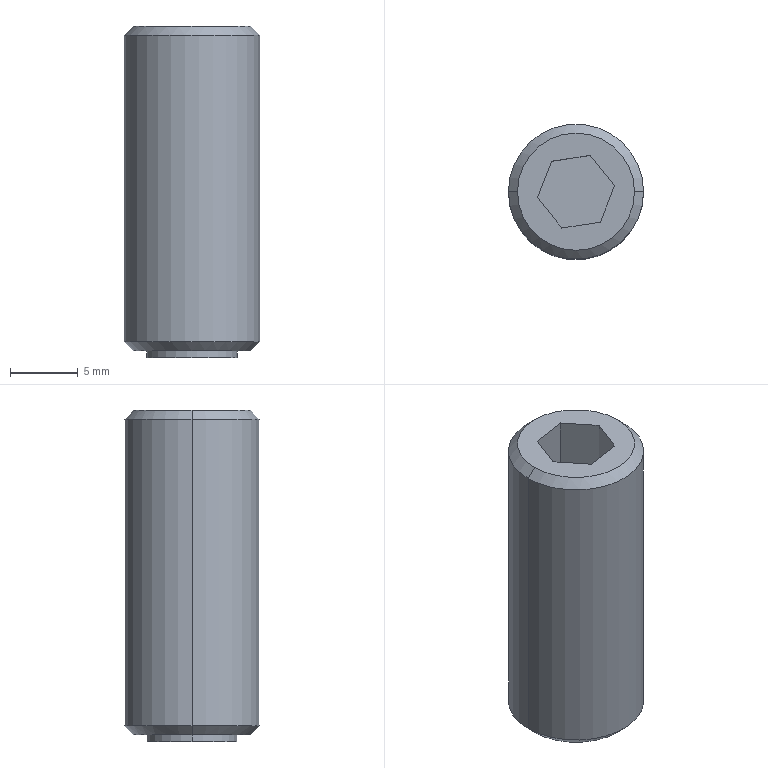Part | NX | 1 solid | 18 faces | box 10 x 10 x 24.5 mm | volume 1781 mm3 | plane 10 | cylinder 4 | cone 4 | commonest cylinder face diameters 6.667 x2 10 x2
STEP:
#1=CARTESIAN_POINT('',(3.333,0.,-12.5));
#2=VERTEX_POINT('',#1);
#3=CARTESIAN_POINT('',(-3.333,0.,-12.5));
#4=VERTEX_POINT('',#3);
#5=CARTESIAN_POINT('',(0.,0.,-12.5));
#6=DIRECTION('',(0.,0.,-1.));
#7=DIRECTION('',(-1.,0.,0.));
#8=AXIS2_PLACEMENT_3D('',#5,#6,#7);
#9=CIRCLE('',#8,3.333);
#10=EDGE_CURVE('',#2,#4,#9,.T.);
#11=ORIENTED_EDGE('',*,*,#10,.F.);
#12=CARTESIAN_POINT('',(3.333,0.,-12.));
#13=VERTEX_POINT('',#12);
#14=CARTESIAN_POINT('',(3.333,0.,-12.5));
#15=DIRECTION('',(0.,0.,1.));
#16=VECTOR('',#15,1000.);
#17=LINE('',#14,#16);
#18=EDGE_CURVE('',#2,#13,#17,.T.);
#19=ORIENTED_EDGE('',*,*,#18,.T.);
#20=CARTESIAN_POINT('',(-3.333,0.,-12.));
#21=VERTEX_POINT('',#20);
#22=CARTESIAN_POINT('',(0.,0.,-12.));
#23=DIRECTION('',(0.,0.,-1.));
#24=DIRECTION('',(1.,0.,0.));
#25=AXIS2_PLACEMENT_3D('',#22,#23,#24);
#26=CIRCLE('',#25,3.333);
#27=EDGE_CURVE('',#13,#21,#26,.T.);
#28=ORIENTED_EDGE('',*,*,#27,.T.);
#29=CARTESIAN_POINT('',(-3.333,0.,-12.5));
#30=DIRECTION('',(0.,0.,1.));
#31=VECTOR('',#30,1000.);
#32=LINE('',#29,#31);
#33=EDGE_CURVE('',#4,#21,#32,.T.);
#34=ORIENTED_EDGE('',*,*,#33,.F.);
#35=EDGE_LOOP('',(#11,#19,#28,#34));
#36=FACE_BOUND('',#35,.T.);
#37=CARTESIAN_POINT('',(0.,0.,-12.5));
#38=DIRECTION('',(0.,0.,1.));
#39=DIRECTION('',(1.,0.,0.));
#40=AXIS2_PLACEMENT_3D('',#37,#38,#39);
#41=CYLINDRICAL_SURFACE('',#40,3.333);
#42=ADVANCED_FACE('',(#36),#41,.T.);
#43=CARTESIAN_POINT('',(5.,0.,-11.333));
#44=VERTEX_POINT('',#43);
#45=CARTESIAN_POINT('',(-5.,0.,-11.333));
#46=VERTEX_POINT('',#45);
#47=CARTESIAN_POINT('',(0.,0.,-11.333));
#48=DIRECTION('',(0.,0.,1.));
#49=DIRECTION('',(1.,0.,0.));
#50=AXIS2_PLACEMENT_3D('',#47,#48,#49);
#51=CIRCLE('',#50,5.);
#52=EDGE_CURVE('',#44,#46,#51,.T.);
#53=ORIENTED_EDGE('',*,*,#52,.F.);
#54=CARTESIAN_POINT('',(4.333,0.,-12.));
#55=VERTEX_POINT('',#54);
#56=CARTESIAN_POINT('',(5.,0.,-11.333));
#57=DIRECTION('',(0.7071,0.,0.7071));
#58=VECTOR('',#57,1000.);
#59=LINE('',#56,#58);
#60=EDGE_CURVE('',#55,#44,#59,.T.);
#61=ORIENTED_EDGE('',*,*,#60,.F.);
#62=CARTESIAN_POINT('',(-4.333,0.,-12.));
#63=VERTEX_POINT('',#62);
#64=CARTESIAN_POINT('',(0.,0.,-12.));
#65=DIRECTION('',(0.,0.,-1.));
#66=DIRECTION('',(1.,0.,0.));
#67=AXIS2_PLACEMENT_3D('',#64,#65,#66);
#68=CIRCLE('',#67,4.333);
#69=EDGE_CURVE('',#63,#55,#68,.T.);
#70=ORIENTED_EDGE('',*,*,#69,.F.);
#71=CARTESIAN_POINT('',(-5.,0.,-11.333));
#72=DIRECTION('',(-0.7071,0.,0.7071));
#73=VECTOR('',#72,1000.);
#74=LINE('',#71,#73);
#75=EDGE_CURVE('',#63,#46,#74,.T.);
#76=ORIENTED_EDGE('',*,*,#75,.T.);
#77=EDGE_LOOP('',(#53,#61,#70,#76));
#78=FACE_BOUND('',#77,.T.);
#79=CARTESIAN_POINT('',(0.,0.,-11.333));
#80=DIRECTION('',(0.,0.,1.));
#81=DIRECTION('',(1.,0.,0.));
#82=AXIS2_PLACEMENT_3D('',#79,#80,#81);
#83=CONICAL_SURFACE('',#82,5.,0.7854);
#84=ADVANCED_FACE('',(#78),#83,.T.);
#85=CARTESIAN_POINT('',(4.333,0.,12.));
#86=VERTEX_POINT('',#85);
#87=CARTESIAN_POINT('',(-4.333,0.,12.));
#88=VERTEX_POINT('',#87);
#89=CARTESIAN_POINT('',(0.,0.,12.));
#90=DIRECTION('',(0.,0.,1.));
#91=DIRECTION('',(1.,0.,0.));
#92=AXIS2_PLACEMENT_3D('',#89,#90,#91);
#93=CIRCLE('',#92,4.333);
#94=EDGE_CURVE('',#86,#88,#93,.T.);
#95=ORIENTED_EDGE('',*,*,#94,.F.);
#96=CARTESIAN_POINT('',(5.,0.,11.333));
#97=VERTEX_POINT('',#96);
#98=CARTESIAN_POINT('',(4.333,0.,12.));
#99=DIRECTION('',(0.7071,0.,-0.7071));
#100=VECTOR('',#99,1000.);
#101=LINE('',#98,#100);
#102=EDGE_CURVE('',#86,#97,#101,.T.);
#103=ORIENTED_EDGE('',*,*,#102,.T.);
#104=CARTESIAN_POINT('',(-5.,0.,11.333));
#105=VERTEX_POINT('',#104);
#106=CARTESIAN_POINT('',(0.,0.,11.333));
#107=DIRECTION('',(0.,0.,-1.));
#108=DIRECTION('',(1.,0.,0.));
#109=AXIS2_PLACEMENT_3D('',#106,#107,#108);
#110=CIRCLE('',#109,5.);
#111=EDGE_CURVE('',#105,#97,#110,.T.);
#112=ORIENTED_EDGE('',*,*,#111,.F.);
#113=CARTESIAN_POINT('',(-4.333,0.,12.));
#114=DIRECTION('',(-0.7071,0.,-0.7071));
#115=VECTOR('',#114,1000.);
#116=LINE('',#113,#115);
#117=EDGE_CURVE('',#88,#105,#116,.T.);
#118=ORIENTED_EDGE('',*,*,#117,.F.);
#119=EDGE_LOOP('',(#95,#103,#112,#118));
#120=FACE_BOUND('',#119,.T.);
#121=CARTESIAN_POINT('',(0.,0.,12.));
#122=DIRECTION('',(0.,0.,-1.));
#123=DIRECTION('',(-1.,0.,0.));
#124=AXIS2_PLACEMENT_3D('',#121,#122,#123);
#125=CONICAL_SURFACE('',#124,4.333,0.7854);
#126=ADVANCED_FACE('',(#120),#125,.T.);
#127=CARTESIAN_POINT('',(0.,0.,11.333));
#128=DIRECTION('',(0.,0.,-1.));
#129=DIRECTION('',(1.,0.,0.));
#130=AXIS2_PLACEMENT_3D('',#127,#128,#129);
#131=CIRCLE('',#130,5.);
#132=EDGE_CURVE('',#97,#105,#131,.T.);
#133=ORIENTED_EDGE('',*,*,#132,.T.);
#134=CARTESIAN_POINT('',(-5.,0.,12.));
#135=DIRECTION('',(0.,0.,-1.));
#136=VECTOR('',#135,1000.);
#137=LINE('',#134,#136);
#138=EDGE_CURVE('',#46,#105,#137,.F.);
#139=ORIENTED_EDGE('',*,*,#138,.F.);
#140=CARTESIAN_POINT('',(0.,0.,-11.333));
#141=DIRECTION('',(0.,0.,1.));
#142=DIRECTION('',(1.,0.,0.));
#143=AXIS2_PLACEMENT_3D('',#140,#141,#142);
#144=CIRCLE('',#143,5.);
#145=EDGE_CURVE('',#46,#44,#144,.T.);
#146=ORIENTED_EDGE('',*,*,#145,.T.);
#147=CARTESIAN_POINT('',(5.,0.,12.));
#148=DIRECTION('',(0.,0.,-1.));
#149=VECTOR('',#148,1000.);
#150=LINE('',#147,#149);
#151=EDGE_CURVE('',#44,#97,#150,.F.);
#152=ORIENTED_EDGE('',*,*,#151,.T.);
#153=EDGE_LOOP('',(#133,#139,#146,#152));
#154=FACE_BOUND('',#153,.T.);
#155=CARTESIAN_POINT('',(0.,0.,12.));
#156=DIRECTION('',(0.,0.,-1.));
#157=DIRECTION('',(-1.,0.,0.));
#158=AXIS2_PLACEMENT_3D('',#155,#156,#157);
#159=CYLINDRICAL_SURFACE('',#158,5.);
#160=ADVANCED_FACE('',(#154),#159,.T.);
#161=ORIENTED_EDGE('',*,*,#69,.T.);
#162=CARTESIAN_POINT('',(0.,0.,-12.));
#163=DIRECTION('',(0.,0.,-1.));
#164=DIRECTION('',(1.,0.,0.));
#165=AXIS2_PLACEMENT_3D('',#162,#163,#164);
#166=CIRCLE('',#165,4.333);
#167=EDGE_CURVE('',#55,#63,#166,.T.);
#168=ORIENTED_EDGE('',*,*,#167,.T.);
#169=EDGE_LOOP('',(#161,#168));
#170=FACE_BOUND('',#169,.T.);
#171=CARTESIAN_POINT('',(0.,0.,-12.));
#172=DIRECTION('',(0.,0.,-1.));
#173=DIRECTION('',(1.,0.,0.));
#174=AXIS2_PLACEMENT_3D('',#171,#172,#173);
#175=CIRCLE('',#174,3.333);
#176=EDGE_CURVE('',#21,#13,#175,.T.);
#177=ORIENTED_EDGE('',*,*,#176,.F.);
#178=ORIENTED_EDGE('',*,*,#27,.F.);
#179=EDGE_LOOP('',(#177,#178));
#180=FACE_BOUND('',#179,.T.);
#181=CARTESIAN_POINT('',(0.,0.,-12.));
#182=DIRECTION('',(0.,0.,1.));
#183=DIRECTION('',(1.,0.,0.));
#184=AXIS2_PLACEMENT_3D('',#181,#182,#183);
#185=PLANE('',#184);
#186=ADVANCED_FACE('',(#170,#180),#185,.F.);
#187=CARTESIAN_POINT('',(-1.047,-2.69,7.));
#188=VERTEX_POINT('',#187);
#189=CARTESIAN_POINT('',(1.806,-2.252,7.));
#190=VERTEX_POINT('',#189);
#191=CARTESIAN_POINT('',(-1.047,-2.69,7.));
#192=DIRECTION('',(0.9884,0.1519,0.));
#193=VECTOR('',#192,1000.);
#194=LINE('',#191,#193);
#195=EDGE_CURVE('',#188,#190,#194,.T.);
#196=ORIENTED_EDGE('',*,*,#195,.T.);
#197=CARTESIAN_POINT('',(2.853,0.4385,7.));
#198=VERTEX_POINT('',#197);
#199=CARTESIAN_POINT('',(1.806,-2.252,7.));
#200=DIRECTION('',(0.3627,0.9319,0.));
#201=VECTOR('',#200,1000.);
#202=LINE('',#199,#201);
#203=EDGE_CURVE('',#190,#198,#202,.T.);
#204=ORIENTED_EDGE('',*,*,#203,.T.);
#205=CARTESIAN_POINT('',(1.047,2.69,7.));
#206=VERTEX_POINT('',#205);
#207=CARTESIAN_POINT('',(2.853,0.4385,7.));
#208=DIRECTION('',(-0.6257,0.78,0.));
#209=VECTOR('',#208,1000.);
#210=LINE('',#207,#209);
#211=EDGE_CURVE('',#198,#206,#210,.T.);
#212=ORIENTED_EDGE('',*,*,#211,.T.);
#213=CARTESIAN_POINT('',(-1.806,2.252,7.));
#214=VERTEX_POINT('',#213);
#215=CARTESIAN_POINT('',(1.047,2.69,7.));
#216=DIRECTION('',(-0.9884,-0.1519,0.));
#217=VECTOR('',#216,1000.);
#218=LINE('',#215,#217);
#219=EDGE_CURVE('',#206,#214,#218,.T.);
#220=ORIENTED_EDGE('',*,*,#219,.T.);
#221=CARTESIAN_POINT('',(-2.853,-0.4385,7.));
#222=VERTEX_POINT('',#221);
#223=CARTESIAN_POINT('',(-1.806,2.252,7.));
#224=DIRECTION('',(-0.3627,-0.9319,0.));
#225=VECTOR('',#224,1000.);
#226=LINE('',#223,#225);
#227=EDGE_CURVE('',#214,#222,#226,.T.);
#228=ORIENTED_EDGE('',*,*,#227,.T.);
#229=CARTESIAN_POINT('',(-2.853,-0.4385,7.));
#230=DIRECTION('',(0.6257,-0.78,0.));
#231=VECTOR('',#230,1000.);
#232=LINE('',#229,#231);
#233=EDGE_CURVE('',#222,#188,#232,.T.);
#234=ORIENTED_EDGE('',*,*,#233,.T.);
#235=EDGE_LOOP('',(#196,#204,#212,#220,#228,#234));
#236=FACE_BOUND('',#235,.T.);
#237=CARTESIAN_POINT('',(1.806,-2.252,7.));
#238=DIRECTION('',(0.,0.,1.));
#239=DIRECTION('',(1.,0.,0.));
#240=AXIS2_PLACEMENT_3D('',#237,#238,#239);
#241=PLANE('',#240);
#242=ADVANCED_FACE('',(#236),#241,.T.);
#243=ORIENTED_EDGE('',*,*,#94,.T.);
#244=CARTESIAN_POINT('',(0.,0.,12.));
#245=DIRECTION('',(0.,0.,1.));
#246=DIRECTION('',(1.,0.,0.));
#247=AXIS2_PLACEMENT_3D('',#244,#245,#246);
#248=CIRCLE('',#247,4.333);
#249=EDGE_CURVE('',#88,#86,#248,.T.);
#250=ORIENTED_EDGE('',*,*,#249,.T.);
#251=EDGE_LOOP('',(#243,#250));
#252=FACE_BOUND('',#251,.T.);
#253=CARTESIAN_POINT('',(-1.047,-2.69,12.));
#254=VERTEX_POINT('',#253);
#255=CARTESIAN_POINT('',(1.806,-2.252,12.));
#256=VERTEX_POINT('',#255);
#257=CARTESIAN_POINT('',(-1.047,-2.69,12.));
#258=DIRECTION('',(0.9884,0.1519,0.));
#259=VECTOR('',#258,1000.);
#260=LINE('',#257,#259);
#261=EDGE_CURVE('',#254,#256,#260,.T.);
#262=ORIENTED_EDGE('',*,*,#261,.F.);
#263=CARTESIAN_POINT('',(-2.853,-0.4385,12.));
#264=VERTEX_POINT('',#263);
#265=CARTESIAN_POINT('',(-2.853,-0.4385,12.));
#266=DIRECTION('',(0.6257,-0.78,0.));
#267=VECTOR('',#266,1000.);
#268=LINE('',#265,#267);
#269=EDGE_CURVE('',#264,#254,#268,.T.);
#270=ORIENTED_EDGE('',*,*,#269,.F.);
#271=CARTESIAN_POINT('',(-1.806,2.252,12.));
#272=VERTEX_POINT('',#271);
#273=CARTESIAN_POINT('',(-1.806,2.252,12.));
#274=DIRECTION('',(-0.3627,-0.9319,0.));
#275=VECTOR('',#274,1000.);
#276=LINE('',#273,#275);
#277=EDGE_CURVE('',#272,#264,#276,.T.);
#278=ORIENTED_EDGE('',*,*,#277,.F.);
#279=CARTESIAN_POINT('',(1.047,2.69,12.));
#280=VERTEX_POINT('',#279);
#281=CARTESIAN_POINT('',(1.047,2.69,12.));
#282=DIRECTION('',(-0.9884,-0.1519,0.));
#283=VECTOR('',#282,1000.);
#284=LINE('',#281,#283);
#285=EDGE_CURVE('',#280,#272,#284,.T.);
#286=ORIENTED_EDGE('',*,*,#285,.F.);
#287=CARTESIAN_POINT('',(2.853,0.4385,12.));
#288=VERTEX_POINT('',#287);
#289=CARTESIAN_POINT('',(2.853,0.4385,12.));
#290=DIRECTION('',(-0.6257,0.78,0.));
#291=VECTOR('',#290,1000.);
#292=LINE('',#289,#291);
#293=EDGE_CURVE('',#288,#280,#292,.T.);
#294=ORIENTED_EDGE('',*,*,#293,.F.);
#295=CARTESIAN_POINT('',(1.806,-2.252,12.));
#296=DIRECTION('',(0.3627,0.9319,0.));
#297=VECTOR('',#296,1000.);
#298=LINE('',#295,#297);
#299=EDGE_CURVE('',#256,#288,#298,.T.);
#300=ORIENTED_EDGE('',*,*,#299,.F.);
#301=EDGE_LOOP('',(#262,#270,#278,#286,#294,#300));
#302=FACE_BOUND('',#301,.T.);
#303=CARTESIAN_POINT('',(0.,0.,12.));
#304=DIRECTION('',(0.,0.,1.));
#305=DIRECTION('',(1.,0.,0.));
#306=AXIS2_PLACEMENT_3D('',#303,#304,#305);
#307=PLANE('',#306);
#308=ADVANCED_FACE('',(#252,#302),#307,.T.);
#309=ORIENTED_EDGE('',*,*,#10,.T.);
#310=CARTESIAN_POINT('',(0.,0.,-12.5));
#311=DIRECTION('',(0.,0.,-1.));
#312=DIRECTION('',(-1.,0.,0.));
#313=AXIS2_PLACEMENT_3D('',#310,#311,#312);
#314=CIRCLE('',#313,3.333);
#315=EDGE_CURVE('',#4,#2,#314,.T.);
#316=ORIENTED_EDGE('',*,*,#315,.T.);
#317=EDGE_LOOP('',(#309,#316));
#318=FACE_BOUND('',#317,.T.);
#319=CARTESIAN_POINT('',(0.,0.,-12.5));
#320=DIRECTION('',(0.,0.,-1.));
#321=DIRECTION('',(0.,-1.,0.));
#322=AXIS2_PLACEMENT_3D('',#319,#320,#321);
#323=PLANE('',#322);
#324=ADVANCED_FACE('',(#318),#323,.T.);
#325=ORIENTED_EDGE('',*,*,#299,.T.);
#326=CARTESIAN_POINT('',(2.853,0.4385,7.));
#327=DIRECTION('',(0.,0.,1.));
#328=VECTOR('',#327,1000.);
#329=LINE('',#326,#328);
#330=EDGE_CURVE('',#198,#288,#329,.T.);
#331=ORIENTED_EDGE('',*,*,#330,.F.);
#332=ORIENTED_EDGE('',*,*,#203,.F.);
#333=CARTESIAN_POINT('',(1.806,-2.252,7.));
#334=DIRECTION('',(0.,0.,1.));
#335=VECTOR('',#334,1000.);
#336=LINE('',#333,#335);
#337=EDGE_CURVE('',#190,#256,#336,.T.);
#338=ORIENTED_EDGE('',*,*,#337,.T.);
#339=EDGE_LOOP('',(#325,#331,#332,#338));
#340=FACE_BOUND('',#339,.T.);
#341=CARTESIAN_POINT('',(1.806,-2.252,7.));
#342=DIRECTION('',(0.9319,-0.3627,0.));
#343=DIRECTION('',(0.,0.,-1.));
#344=AXIS2_PLACEMENT_3D('',#341,#342,#343);
#345=PLANE('',#344);
#346=ADVANCED_FACE('',(#340),#345,.F.);
#347=ORIENTED_EDGE('',*,*,#261,.T.);
#348=ORIENTED_EDGE('',*,*,#337,.F.);
#349=ORIENTED_EDGE('',*,*,#195,.F.);
#350=CARTESIAN_POINT('',(-1.047,-2.69,7.));
#351=DIRECTION('',(0.,0.,1.));
#352=VECTOR('',#351,1000.);
#353=LINE('',#350,#352);
#354=EDGE_CURVE('',#188,#254,#353,.T.);
#355=ORIENTED_EDGE('',*,*,#354,.T.);
#356=EDGE_LOOP('',(#347,#348,#349,#355));
#357=FACE_BOUND('',#356,.T.);
#358=CARTESIAN_POINT('',(-1.047,-2.69,7.));
#359=DIRECTION('',(0.1519,-0.9884,0.));
#360=DIRECTION('',(0.,0.,-1.));
#361=AXIS2_PLACEMENT_3D('',#358,#359,#360);
#362=PLANE('',#361);
#363=ADVANCED_FACE('',(#357),#362,.F.);
#364=ORIENTED_EDGE('',*,*,#269,.T.);
#365=ORIENTED_EDGE('',*,*,#354,.F.);
#366=ORIENTED_EDGE('',*,*,#233,.F.);
#367=CARTESIAN_POINT('',(-2.853,-0.4385,7.));
#368=DIRECTION('',(0.,0.,1.));
#369=VECTOR('',#368,1000.);
#370=LINE('',#367,#369);
#371=EDGE_CURVE('',#222,#264,#370,.T.);
#372=ORIENTED_EDGE('',*,*,#371,.T.);
#373=EDGE_LOOP('',(#364,#365,#366,#372));
#374=FACE_BOUND('',#373,.T.);
#375=CARTESIAN_POINT('',(-2.853,-0.4385,7.));
#376=DIRECTION('',(-0.78,-0.6257,0.));
#377=DIRECTION('',(-0.6257,0.78,0.));
#378=AXIS2_PLACEMENT_3D('',#375,#376,#377);
#379=PLANE('',#378);
#380=ADVANCED_FACE('',(#374),#379,.F.);
#381=ORIENTED_EDGE('',*,*,#277,.T.);
#382=ORIENTED_EDGE('',*,*,#371,.F.);
#383=ORIENTED_EDGE('',*,*,#227,.F.);
#384=CARTESIAN_POINT('',(-1.806,2.252,7.));
#385=DIRECTION('',(0.,0.,1.));
#386=VECTOR('',#385,1000.);
#387=LINE('',#384,#386);
#388=EDGE_CURVE('',#214,#272,#387,.T.);
#389=ORIENTED_EDGE('',*,*,#388,.T.);
#390=EDGE_LOOP('',(#381,#382,#383,#389));
#391=FACE_BOUND('',#390,.T.);
#392=CARTESIAN_POINT('',(-1.806,2.252,7.));
#393=DIRECTION('',(-0.9319,0.3627,0.));
#394=DIRECTION('',(0.,0.,1.));
#395=AXIS2_PLACEMENT_3D('',#392,#393,#394);
#396=PLANE('',#395);
#397=ADVANCED_FACE('',(#391),#396,.F.);
#398=ORIENTED_EDGE('',*,*,#285,.T.);
#399=ORIENTED_EDGE('',*,*,#388,.F.);
#400=ORIENTED_EDGE('',*,*,#219,.F.);
#401=CARTESIAN_POINT('',(1.047,2.69,7.));
#402=DIRECTION('',(0.,0.,1.));
#403=VECTOR('',#402,1000.);
#404=LINE('',#401,#403);
#405=EDGE_CURVE('',#206,#280,#404,.T.);
#406=ORIENTED_EDGE('',*,*,#405,.T.);
#407=EDGE_LOOP('',(#398,#399,#400,#406));
#408=FACE_BOUND('',#407,.T.);
#409=CARTESIAN_POINT('',(1.047,2.69,7.));
#410=DIRECTION('',(-0.1519,0.9884,0.));
#411=DIRECTION('',(0.,0.,1.));
#412=AXIS2_PLACEMENT_3D('',#409,#410,#411);
#413=PLANE('',#412);
#414=ADVANCED_FACE('',(#408),#413,.F.);
#415=ORIENTED_EDGE('',*,*,#293,.T.);
#416=ORIENTED_EDGE('',*,*,#405,.F.);
#417=ORIENTED_EDGE('',*,*,#211,.F.);
#418=ORIENTED_EDGE('',*,*,#330,.T.);
#419=EDGE_LOOP('',(#415,#416,#417,#418));
#420=FACE_BOUND('',#419,.T.);
#421=CARTESIAN_POINT('',(2.853,0.4385,7.));
#422=DIRECTION('',(0.78,0.6257,0.));
#423=DIRECTION('',(0.,0.,-1.));
#424=AXIS2_PLACEMENT_3D('',#421,#422,#423);
#425=PLANE('',#424);
#426=ADVANCED_FACE('',(#420),#425,.F.);
#427=ORIENTED_EDGE('',*,*,#52,.T.);
#428=ORIENTED_EDGE('',*,*,#138,.T.);
#429=ORIENTED_EDGE('',*,*,#111,.T.);
#430=ORIENTED_EDGE('',*,*,#151,.F.);
#431=EDGE_LOOP('',(#427,#428,#429,#430));
#432=FACE_BOUND('',#431,.T.);
#433=CARTESIAN_POINT('',(0.,0.,12.));
#434=DIRECTION('',(0.,0.,-1.));
#435=DIRECTION('',(-1.,0.,0.));
#436=AXIS2_PLACEMENT_3D('',#433,#434,#435);
#437=CYLINDRICAL_SURFACE('',#436,5.);
#438=ADVANCED_FACE('',(#432),#437,.T.);
#439=ORIENTED_EDGE('',*,*,#60,.T.);
#440=ORIENTED_EDGE('',*,*,#145,.F.);
#441=ORIENTED_EDGE('',*,*,#75,.F.);
#442=ORIENTED_EDGE('',*,*,#167,.F.);
#443=EDGE_LOOP('',(#439,#440,#441,#442));
#444=FACE_BOUND('',#443,.T.);
#445=CARTESIAN_POINT('',(0.,0.,-11.333));
#446=DIRECTION('',(0.,0.,1.));
#447=DIRECTION('',(1.,0.,0.));
#448=AXIS2_PLACEMENT_3D('',#445,#446,#447);
#449=CONICAL_SURFACE('',#448,5.,0.7854);
#450=ADVANCED_FACE('',(#444),#449,.T.);
#451=ORIENTED_EDGE('',*,*,#176,.T.);
#452=ORIENTED_EDGE('',*,*,#18,.F.);
#453=ORIENTED_EDGE('',*,*,#315,.F.);
#454=ORIENTED_EDGE('',*,*,#33,.T.);
#455=EDGE_LOOP('',(#451,#452,#453,#454));
#456=FACE_BOUND('',#455,.T.);
#457=CARTESIAN_POINT('',(0.,0.,-12.5));
#458=DIRECTION('',(0.,0.,1.));
#459=DIRECTION('',(1.,0.,0.));
#460=AXIS2_PLACEMENT_3D('',#457,#458,#459);
#461=CYLINDRICAL_SURFACE('',#460,3.333);
#462=ADVANCED_FACE('',(#456),#461,.T.);
#463=ORIENTED_EDGE('',*,*,#132,.F.);
#464=ORIENTED_EDGE('',*,*,#102,.F.);
#465=ORIENTED_EDGE('',*,*,#249,.F.);
#466=ORIENTED_EDGE('',*,*,#117,.T.);
#467=EDGE_LOOP('',(#463,#464,#465,#466));
#468=FACE_BOUND('',#467,.T.);
#469=CARTESIAN_POINT('',(0.,0.,12.));
#470=DIRECTION('',(0.,0.,-1.));
#471=DIRECTION('',(-1.,0.,0.));
#472=AXIS2_PLACEMENT_3D('',#469,#470,#471);
#473=CONICAL_SURFACE('',#472,4.333,0.7854);
#474=ADVANCED_FACE('',(#468),#473,.T.);
#475=CLOSED_SHELL('',(#42,#84,#126,#160,#186,#242,#308,#324,#346,#363,#380,#397,#414,#426,#438,#450,#462,#474));
#476=MANIFOLD_SOLID_BREP('',#475);
#477=(LENGTH_UNIT()NAMED_UNIT(*)SI_UNIT(.MILLI.,.METRE.));
#478=UNCERTAINTY_MEASURE_WITH_UNIT(LENGTH_MEASURE(0.00001),#477,'','');
#479=(NAMED_UNIT(*)PLANE_ANGLE_UNIT()SI_UNIT($,.RADIAN.));
#480=(NAMED_UNIT(*)SI_UNIT($,.STERADIAN.)SOLID_ANGLE_UNIT());
#481=(GEOMETRIC_REPRESENTATION_CONTEXT(3)GLOBAL_UNCERTAINTY_ASSIGNED_CONTEXT((#478))GLOBAL_UNIT_ASSIGNED_CONTEXT((#477,#479,#480))REPRESENTATION_CONTEXT('',''));
#482=ADVANCED_BREP_SHAPE_REPRESENTATION('',(#476),#481);